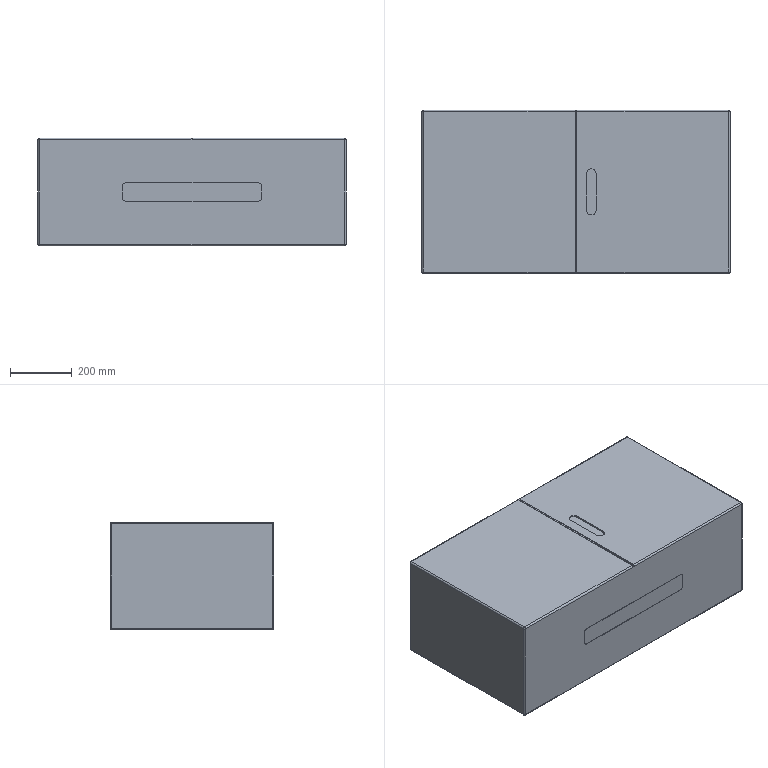Part | SolidWorks | features ICE 3, Fillet 2, Cut 1, Extrusion 1 | 1 solid | 44 faces | box 1000 x 530 x 350 mm | volume 185406118 mm3 | plane 18 | cylinder 18 | sphere 8 | commonest cylinder face diameters 10 x12 20 x4 30 x2
STEP:
#1=CARTESIAN_POINT('',(35.,60.,350.));
#2=VERTEX_POINT('',#1);
#3=CARTESIAN_POINT('',(35.,-60.,350.));
#4=VERTEX_POINT('',#3);
#5=CARTESIAN_POINT('',(35.,60.,350.));
#6=DIRECTION('',(0.,-1.,0.));
#7=VECTOR('',#6,1000.);
#8=LINE('',#5,#7);
#9=EDGE_CURVE('',#2,#4,#8,.T.);
#10=ORIENTED_EDGE('',*,*,#9,.F.);
#11=CARTESIAN_POINT('',(65.,60.,350.));
#12=VERTEX_POINT('',#11);
#13=CARTESIAN_POINT('',(50.,60.,350.));
#14=DIRECTION('',(0.,0.,1.));
#15=DIRECTION('',(1.,0.,0.));
#16=AXIS2_PLACEMENT_3D('',#13,#14,#15);
#17=CIRCLE('',#16,15.);
#18=EDGE_CURVE('',#12,#2,#17,.T.);
#19=ORIENTED_EDGE('',*,*,#18,.F.);
#20=CARTESIAN_POINT('',(65.,-60.,350.));
#21=VERTEX_POINT('',#20);
#22=CARTESIAN_POINT('',(65.,60.,350.));
#23=DIRECTION('',(0.,1.,0.));
#24=VECTOR('',#23,1000.);
#25=LINE('',#22,#24);
#26=EDGE_CURVE('',#21,#12,#25,.T.);
#27=ORIENTED_EDGE('',*,*,#26,.F.);
#28=CARTESIAN_POINT('',(50.,-60.,350.));
#29=DIRECTION('',(0.,0.,1.));
#30=DIRECTION('',(1.,0.,0.));
#31=AXIS2_PLACEMENT_3D('',#28,#29,#30);
#32=CIRCLE('',#31,15.);
#33=EDGE_CURVE('',#4,#21,#32,.T.);
#34=ORIENTED_EDGE('',*,*,#33,.F.);
#35=EDGE_LOOP('',(#10,#19,#27,#34));
#36=FACE_BOUND('',#35,.T.);
#37=CARTESIAN_POINT('',(495.,260.,350.));
#38=VERTEX_POINT('',#37);
#39=CARTESIAN_POINT('',(2.5,260.,350.));
#40=VERTEX_POINT('',#39);
#41=CARTESIAN_POINT('',(500.,260.,350.));
#42=DIRECTION('',(-1.,0.,0.));
#43=VECTOR('',#42,1000.);
#44=LINE('',#41,#43);
#45=EDGE_CURVE('',#38,#40,#44,.T.);
#46=ORIENTED_EDGE('',*,*,#45,.T.);
#47=CARTESIAN_POINT('',(2.5,-260.,350.));
#48=VERTEX_POINT('',#47);
#49=CARTESIAN_POINT('',(2.5,-265.,350.));
#50=DIRECTION('',(0.,1.,0.));
#51=VECTOR('',#50,1000.);
#52=LINE('',#49,#51);
#53=EDGE_CURVE('',#48,#40,#52,.T.);
#54=ORIENTED_EDGE('',*,*,#53,.F.);
#55=CARTESIAN_POINT('',(495.,-260.,350.));
#56=VERTEX_POINT('',#55);
#57=CARTESIAN_POINT('',(500.,-260.,350.));
#58=DIRECTION('',(1.,0.,0.));
#59=VECTOR('',#58,1000.);
#60=LINE('',#57,#59);
#61=EDGE_CURVE('',#48,#56,#60,.T.);
#62=ORIENTED_EDGE('',*,*,#61,.T.);
#63=CARTESIAN_POINT('',(495.,265.,350.));
#64=DIRECTION('',(0.,1.,0.));
#65=VECTOR('',#64,1000.);
#66=LINE('',#63,#65);
#67=EDGE_CURVE('',#56,#38,#66,.T.);
#68=ORIENTED_EDGE('',*,*,#67,.T.);
#69=EDGE_LOOP('',(#46,#54,#62,#68));
#70=FACE_OUTER_BOUND('',#69,.T.);
#71=CARTESIAN_POINT('',(500.,265.,350.));
#72=DIRECTION('',(0.,0.,-1.));
#73=DIRECTION('',(-1.,0.,0.));
#74=AXIS2_PLACEMENT_3D('',#71,#72,#73);
#75=PLANE('',#74);
#76=ADVANCED_FACE('',(#36,#70),#75,.F.);
#77=CARTESIAN_POINT('',(500.,-260.,5.));
#78=VERTEX_POINT('',#77);
#79=CARTESIAN_POINT('',(500.,260.,5.));
#80=VERTEX_POINT('',#79);
#81=CARTESIAN_POINT('',(500.,265.,5.));
#82=DIRECTION('',(0.,1.,0.));
#83=VECTOR('',#82,1000.);
#84=LINE('',#81,#83);
#85=EDGE_CURVE('',#78,#80,#84,.T.);
#86=ORIENTED_EDGE('',*,*,#85,.T.);
#87=CARTESIAN_POINT('',(500.,260.,345.));
#88=VERTEX_POINT('',#87);
#89=CARTESIAN_POINT('',(500.,260.,350.));
#90=DIRECTION('',(0.,0.,1.));
#91=VECTOR('',#90,1000.);
#92=LINE('',#89,#91);
#93=EDGE_CURVE('',#80,#88,#92,.T.);
#94=ORIENTED_EDGE('',*,*,#93,.T.);
#95=CARTESIAN_POINT('',(500.,-260.,345.));
#96=VERTEX_POINT('',#95);
#97=CARTESIAN_POINT('',(500.,-265.,345.));
#98=DIRECTION('',(0.,-1.,0.));
#99=VECTOR('',#98,1000.);
#100=LINE('',#97,#99);
#101=EDGE_CURVE('',#88,#96,#100,.T.);
#102=ORIENTED_EDGE('',*,*,#101,.T.);
#103=CARTESIAN_POINT('',(500.,-260.,350.));
#104=DIRECTION('',(0.,0.,-1.));
#105=VECTOR('',#104,1000.);
#106=LINE('',#103,#105);
#107=EDGE_CURVE('',#96,#78,#106,.T.);
#108=ORIENTED_EDGE('',*,*,#107,.T.);
#109=EDGE_LOOP('',(#86,#94,#102,#108));
#110=FACE_OUTER_BOUND('',#109,.T.);
#111=CARTESIAN_POINT('',(500.,-265.,350.));
#112=DIRECTION('',(-1.,0.,0.));
#113=DIRECTION('',(0.,0.,1.));
#114=AXIS2_PLACEMENT_3D('',#111,#112,#113);
#115=PLANE('',#114);
#116=ADVANCED_FACE('',(#110),#115,.F.);
#117=CARTESIAN_POINT('',(495.,265.,5.));
#118=VERTEX_POINT('',#117);
#119=CARTESIAN_POINT('',(-495.,265.,5.));
#120=VERTEX_POINT('',#119);
#121=CARTESIAN_POINT('',(-500.,265.,5.));
#122=DIRECTION('',(-1.,0.,0.));
#123=VECTOR('',#122,1000.);
#124=LINE('',#121,#123);
#125=EDGE_CURVE('',#118,#120,#124,.T.);
#126=ORIENTED_EDGE('',*,*,#125,.T.);
#127=CARTESIAN_POINT('',(-495.,265.,345.));
#128=VERTEX_POINT('',#127);
#129=CARTESIAN_POINT('',(-495.,265.,350.));
#130=DIRECTION('',(0.,0.,1.));
#131=VECTOR('',#130,1000.);
#132=LINE('',#129,#131);
#133=EDGE_CURVE('',#120,#128,#132,.T.);
#134=ORIENTED_EDGE('',*,*,#133,.T.);
#135=CARTESIAN_POINT('',(495.,265.,345.));
#136=VERTEX_POINT('',#135);
#137=CARTESIAN_POINT('',(-500.,265.,345.));
#138=DIRECTION('',(1.,0.,0.));
#139=VECTOR('',#138,1000.);
#140=LINE('',#137,#139);
#141=EDGE_CURVE('',#128,#136,#140,.T.);
#142=ORIENTED_EDGE('',*,*,#141,.T.);
#143=CARTESIAN_POINT('',(495.,265.,350.));
#144=DIRECTION('',(0.,0.,-1.));
#145=VECTOR('',#144,1000.);
#146=LINE('',#143,#145);
#147=EDGE_CURVE('',#136,#118,#146,.T.);
#148=ORIENTED_EDGE('',*,*,#147,.T.);
#149=EDGE_LOOP('',(#126,#134,#142,#148));
#150=FACE_OUTER_BOUND('',#149,.T.);
#151=CARTESIAN_POINT('',(-500.,265.,350.));
#152=DIRECTION('',(0.,-1.,0.));
#153=DIRECTION('',(0.,0.,-1.));
#154=AXIS2_PLACEMENT_3D('',#151,#152,#153);
#155=PLANE('',#154);
#156=ADVANCED_FACE('',(#150),#155,.F.);
#157=CARTESIAN_POINT('',(-500.,-260.,345.));
#158=VERTEX_POINT('',#157);
#159=CARTESIAN_POINT('',(-500.,260.,345.));
#160=VERTEX_POINT('',#159);
#161=CARTESIAN_POINT('',(-500.,-265.,345.));
#162=DIRECTION('',(0.,1.,0.));
#163=VECTOR('',#162,1000.);
#164=LINE('',#161,#163);
#165=EDGE_CURVE('',#158,#160,#164,.T.);
#166=ORIENTED_EDGE('',*,*,#165,.T.);
#167=CARTESIAN_POINT('',(-500.,260.,5.));
#168=VERTEX_POINT('',#167);
#169=CARTESIAN_POINT('',(-500.,260.,350.));
#170=DIRECTION('',(0.,0.,-1.));
#171=VECTOR('',#170,1000.);
#172=LINE('',#169,#171);
#173=EDGE_CURVE('',#160,#168,#172,.T.);
#174=ORIENTED_EDGE('',*,*,#173,.T.);
#175=CARTESIAN_POINT('',(-500.,-260.,5.));
#176=VERTEX_POINT('',#175);
#177=CARTESIAN_POINT('',(-500.,-265.,5.));
#178=DIRECTION('',(0.,-1.,0.));
#179=VECTOR('',#178,1000.);
#180=LINE('',#177,#179);
#181=EDGE_CURVE('',#168,#176,#180,.T.);
#182=ORIENTED_EDGE('',*,*,#181,.T.);
#183=CARTESIAN_POINT('',(-500.,-260.,350.));
#184=DIRECTION('',(0.,0.,1.));
#185=VECTOR('',#184,1000.);
#186=LINE('',#183,#185);
#187=EDGE_CURVE('',#176,#158,#186,.T.);
#188=ORIENTED_EDGE('',*,*,#187,.T.);
#189=EDGE_LOOP('',(#166,#174,#182,#188));
#190=FACE_OUTER_BOUND('',#189,.T.);
#191=CARTESIAN_POINT('',(-500.,-265.,350.));
#192=DIRECTION('',(1.,0.,0.));
#193=DIRECTION('',(0.,0.,-1.));
#194=AXIS2_PLACEMENT_3D('',#191,#192,#193);
#195=PLANE('',#194);
#196=ADVANCED_FACE('',(#190),#195,.F.);
#197=CARTESIAN_POINT('',(215.,-265.,205.));
#198=VERTEX_POINT('',#197);
#199=CARTESIAN_POINT('',(-215.,-265.,205.));
#200=VERTEX_POINT('',#199);
#201=CARTESIAN_POINT('',(-225.,-265.,205.));
#202=DIRECTION('',(-1.,0.,0.));
#203=VECTOR('',#202,1000.);
#204=LINE('',#201,#203);
#205=EDGE_CURVE('',#198,#200,#204,.T.);
#206=ORIENTED_EDGE('',*,*,#205,.F.);
#207=CARTESIAN_POINT('',(225.,-265.,195.));
#208=VERTEX_POINT('',#207);
#209=CARTESIAN_POINT('',(215.,-265.,195.));
#210=DIRECTION('',(0.,1.,0.));
#211=DIRECTION('',(0.,0.,1.));
#212=AXIS2_PLACEMENT_3D('',#209,#210,#211);
#213=CIRCLE('',#212,10.);
#214=EDGE_CURVE('',#198,#208,#213,.T.);
#215=ORIENTED_EDGE('',*,*,#214,.T.);
#216=CARTESIAN_POINT('',(225.,-265.,155.));
#217=VERTEX_POINT('',#216);
#218=CARTESIAN_POINT('',(225.,-265.,145.));
#219=DIRECTION('',(0.,0.,1.));
#220=VECTOR('',#219,1000.);
#221=LINE('',#218,#220);
#222=EDGE_CURVE('',#217,#208,#221,.T.);
#223=ORIENTED_EDGE('',*,*,#222,.F.);
#224=CARTESIAN_POINT('',(215.,-265.,145.));
#225=VERTEX_POINT('',#224);
#226=CARTESIAN_POINT('',(215.,-265.,155.));
#227=DIRECTION('',(0.,1.,0.));
#228=DIRECTION('',(0.,0.,1.));
#229=AXIS2_PLACEMENT_3D('',#226,#227,#228);
#230=CIRCLE('',#229,10.);
#231=EDGE_CURVE('',#217,#225,#230,.T.);
#232=ORIENTED_EDGE('',*,*,#231,.T.);
#233=CARTESIAN_POINT('',(-215.,-265.,145.));
#234=VERTEX_POINT('',#233);
#235=CARTESIAN_POINT('',(-225.,-265.,145.));
#236=DIRECTION('',(1.,0.,0.));
#237=VECTOR('',#236,1000.);
#238=LINE('',#235,#237);
#239=EDGE_CURVE('',#234,#225,#238,.T.);
#240=ORIENTED_EDGE('',*,*,#239,.F.);
#241=CARTESIAN_POINT('',(-225.,-265.,155.));
#242=VERTEX_POINT('',#241);
#243=CARTESIAN_POINT('',(-215.,-265.,155.));
#244=DIRECTION('',(0.,1.,0.));
#245=DIRECTION('',(0.,0.,1.));
#246=AXIS2_PLACEMENT_3D('',#243,#244,#245);
#247=CIRCLE('',#246,10.);
#248=EDGE_CURVE('',#234,#242,#247,.T.);
#249=ORIENTED_EDGE('',*,*,#248,.T.);
#250=CARTESIAN_POINT('',(-225.,-265.,195.));
#251=VERTEX_POINT('',#250);
#252=CARTESIAN_POINT('',(-225.,-265.,145.));
#253=DIRECTION('',(0.,0.,-1.));
#254=VECTOR('',#253,1000.);
#255=LINE('',#252,#254);
#256=EDGE_CURVE('',#251,#242,#255,.T.);
#257=ORIENTED_EDGE('',*,*,#256,.F.);
#258=CARTESIAN_POINT('',(-215.,-265.,195.));
#259=DIRECTION('',(0.,1.,0.));
#260=DIRECTION('',(0.,0.,1.));
#261=AXIS2_PLACEMENT_3D('',#258,#259,#260);
#262=CIRCLE('',#261,10.);
#263=EDGE_CURVE('',#251,#200,#262,.T.);
#264=ORIENTED_EDGE('',*,*,#263,.T.);
#265=EDGE_LOOP('',(#206,#215,#223,#232,#240,#249,#257,#264));
#266=FACE_BOUND('',#265,.T.);
#267=CARTESIAN_POINT('',(495.,-265.,345.));
#268=VERTEX_POINT('',#267);
#269=CARTESIAN_POINT('',(-495.,-265.,345.));
#270=VERTEX_POINT('',#269);
#271=CARTESIAN_POINT('',(-500.,-265.,345.));
#272=DIRECTION('',(-1.,0.,0.));
#273=VECTOR('',#272,1000.);
#274=LINE('',#271,#273);
#275=EDGE_CURVE('',#268,#270,#274,.T.);
#276=ORIENTED_EDGE('',*,*,#275,.T.);
#277=CARTESIAN_POINT('',(-495.,-265.,5.));
#278=VERTEX_POINT('',#277);
#279=CARTESIAN_POINT('',(-495.,-265.,350.));
#280=DIRECTION('',(0.,0.,-1.));
#281=VECTOR('',#280,1000.);
#282=LINE('',#279,#281);
#283=EDGE_CURVE('',#270,#278,#282,.T.);
#284=ORIENTED_EDGE('',*,*,#283,.T.);
#285=CARTESIAN_POINT('',(495.,-265.,5.));
#286=VERTEX_POINT('',#285);
#287=CARTESIAN_POINT('',(500.,-265.,5.));
#288=DIRECTION('',(1.,0.,0.));
#289=VECTOR('',#288,1000.);
#290=LINE('',#287,#289);
#291=EDGE_CURVE('',#278,#286,#290,.T.);
#292=ORIENTED_EDGE('',*,*,#291,.T.);
#293=CARTESIAN_POINT('',(495.,-265.,350.));
#294=DIRECTION('',(0.,0.,1.));
#295=VECTOR('',#294,1000.);
#296=LINE('',#293,#295);
#297=EDGE_CURVE('',#286,#268,#296,.T.);
#298=ORIENTED_EDGE('',*,*,#297,.T.);
#299=EDGE_LOOP('',(#276,#284,#292,#298));
#300=FACE_OUTER_BOUND('',#299,.T.);
#301=CARTESIAN_POINT('',(-500.,-265.,350.));
#302=DIRECTION('',(0.,1.,0.));
#303=DIRECTION('',(0.,0.,1.));
#304=AXIS2_PLACEMENT_3D('',#301,#302,#303);
#305=PLANE('',#304);
#306=ADVANCED_FACE('',(#266,#300),#305,.F.);
#307=CARTESIAN_POINT('',(-495.,-260.,350.));
#308=VERTEX_POINT('',#307);
#309=CARTESIAN_POINT('',(-2.5,-260.,350.));
#310=VERTEX_POINT('',#309);
#311=CARTESIAN_POINT('',(500.,-260.,350.));
#312=DIRECTION('',(1.,0.,0.));
#313=VECTOR('',#312,1000.);
#314=LINE('',#311,#313);
#315=EDGE_CURVE('',#308,#310,#314,.T.);
#316=ORIENTED_EDGE('',*,*,#315,.T.);
#317=CARTESIAN_POINT('',(-2.5,260.,350.));
#318=VERTEX_POINT('',#317);
#319=CARTESIAN_POINT('',(-2.5,-265.,350.));
#320=DIRECTION('',(0.,-1.,0.));
#321=VECTOR('',#320,1000.);
#322=LINE('',#319,#321);
#323=EDGE_CURVE('',#318,#310,#322,.T.);
#324=ORIENTED_EDGE('',*,*,#323,.F.);
#325=CARTESIAN_POINT('',(-495.,260.,350.));
#326=VERTEX_POINT('',#325);
#327=CARTESIAN_POINT('',(500.,260.,350.));
#328=DIRECTION('',(-1.,0.,0.));
#329=VECTOR('',#328,1000.);
#330=LINE('',#327,#329);
#331=EDGE_CURVE('',#318,#326,#330,.T.);
#332=ORIENTED_EDGE('',*,*,#331,.T.);
#333=CARTESIAN_POINT('',(-495.,265.,350.));
#334=DIRECTION('',(0.,-1.,0.));
#335=VECTOR('',#334,1000.);
#336=LINE('',#333,#335);
#337=EDGE_CURVE('',#326,#308,#336,.T.);
#338=ORIENTED_EDGE('',*,*,#337,.T.);
#339=EDGE_LOOP('',(#316,#324,#332,#338));
#340=FACE_OUTER_BOUND('',#339,.T.);
#341=CARTESIAN_POINT('',(500.,265.,350.));
#342=DIRECTION('',(0.,0.,-1.));
#343=DIRECTION('',(-1.,0.,0.));
#344=AXIS2_PLACEMENT_3D('',#341,#342,#343);
#345=PLANE('',#344);
#346=ADVANCED_FACE('',(#340),#345,.F.);
#347=CARTESIAN_POINT('',(-495.,-260.,0.));
#348=VERTEX_POINT('',#347);
#349=CARTESIAN_POINT('',(-495.,260.,0.));
#350=VERTEX_POINT('',#349);
#351=CARTESIAN_POINT('',(-495.,265.,0.));
#352=DIRECTION('',(0.,1.,0.));
#353=VECTOR('',#352,1000.);
#354=LINE('',#351,#353);
#355=EDGE_CURVE('',#348,#350,#354,.T.);
#356=ORIENTED_EDGE('',*,*,#355,.T.);
#357=CARTESIAN_POINT('',(495.,260.,0.));
#358=VERTEX_POINT('',#357);
#359=CARTESIAN_POINT('',(500.,260.,0.));
#360=DIRECTION('',(1.,0.,0.));
#361=VECTOR('',#360,1000.);
#362=LINE('',#359,#361);
#363=EDGE_CURVE('',#350,#358,#362,.T.);
#364=ORIENTED_EDGE('',*,*,#363,.T.);
#365=CARTESIAN_POINT('',(495.,-260.,0.));
#366=VERTEX_POINT('',#365);
#367=CARTESIAN_POINT('',(495.,-265.,0.));
#368=DIRECTION('',(0.,-1.,0.));
#369=VECTOR('',#368,1000.);
#370=LINE('',#367,#369);
#371=EDGE_CURVE('',#358,#366,#370,.T.);
#372=ORIENTED_EDGE('',*,*,#371,.T.);
#373=CARTESIAN_POINT('',(-500.,-260.,0.));
#374=DIRECTION('',(-1.,0.,0.));
#375=VECTOR('',#374,1000.);
#376=LINE('',#373,#375);
#377=EDGE_CURVE('',#366,#348,#376,.T.);
#378=ORIENTED_EDGE('',*,*,#377,.T.);
#379=EDGE_LOOP('',(#356,#364,#372,#378));
#380=FACE_OUTER_BOUND('',#379,.T.);
#381=CARTESIAN_POINT('',(500.,265.,0.));
#382=DIRECTION('',(0.,0.,-1.));
#383=DIRECTION('',(-1.,0.,0.));
#384=AXIS2_PLACEMENT_3D('',#381,#382,#383);
#385=PLANE('',#384);
#386=ADVANCED_FACE('',(#380),#385,.T.);
#387=CARTESIAN_POINT('',(2.5,-264.,348.));
#388=VERTEX_POINT('',#387);
#389=CARTESIAN_POINT('',(2.5,-260.,345.));
#390=DIRECTION('',(-1.,0.,0.));
#391=DIRECTION('',(0.,0.,-1.));
#392=AXIS2_PLACEMENT_3D('',#389,#390,#391);
#393=CIRCLE('',#392,5.);
#394=EDGE_CURVE('',#388,#48,#393,.T.);
#395=ORIENTED_EDGE('',*,*,#394,.F.);
#396=CARTESIAN_POINT('',(-2.5,-264.,348.));
#397=VERTEX_POINT('',#396);
#398=CARTESIAN_POINT('',(500.,-264.,348.));
#399=DIRECTION('',(1.,0.,0.));
#400=VECTOR('',#399,1000.);
#401=LINE('',#398,#400);
#402=EDGE_CURVE('',#397,#388,#401,.T.);
#403=ORIENTED_EDGE('',*,*,#402,.F.);
#404=CARTESIAN_POINT('',(-2.5,-260.,345.));
#405=DIRECTION('',(1.,0.,0.));
#406=DIRECTION('',(0.,0.,1.));
#407=AXIS2_PLACEMENT_3D('',#404,#405,#406);
#408=CIRCLE('',#407,5.);
#409=EDGE_CURVE('',#310,#397,#408,.T.);
#410=ORIENTED_EDGE('',*,*,#409,.F.);
#411=ORIENTED_EDGE('',*,*,#315,.F.);
#412=CARTESIAN_POINT('',(-495.,-260.,345.));
#413=DIRECTION('',(-1.,0.,0.));
#414=DIRECTION('',(0.,0.,1.));
#415=AXIS2_PLACEMENT_3D('',#412,#413,#414);
#416=CIRCLE('',#415,5.);
#417=EDGE_CURVE('',#270,#308,#416,.T.);
#418=ORIENTED_EDGE('',*,*,#417,.F.);
#419=ORIENTED_EDGE('',*,*,#275,.F.);
#420=CARTESIAN_POINT('',(495.,-260.,345.));
#421=DIRECTION('',(1.,0.,0.));
#422=DIRECTION('',(0.,0.,-1.));
#423=AXIS2_PLACEMENT_3D('',#420,#421,#422);
#424=CIRCLE('',#423,5.);
#425=EDGE_CURVE('',#56,#268,#424,.T.);
#426=ORIENTED_EDGE('',*,*,#425,.F.);
#427=ORIENTED_EDGE('',*,*,#61,.F.);
#428=EDGE_LOOP('',(#395,#403,#410,#411,#418,#419,#426,#427));
#429=FACE_OUTER_BOUND('',#428,.T.);
#430=CARTESIAN_POINT('',(500.,-260.,345.));
#431=DIRECTION('',(1.,0.,0.));
#432=DIRECTION('',(0.,0.,-1.));
#433=AXIS2_PLACEMENT_3D('',#430,#431,#432);
#434=CYLINDRICAL_SURFACE('',#433,5.);
#435=ADVANCED_FACE('',(#429),#434,.T.);
#436=CARTESIAN_POINT('',(495.,-260.,345.));
#437=DIRECTION('',(0.,1.,0.));
#438=DIRECTION('',(0.,0.,-1.));
#439=AXIS2_PLACEMENT_3D('',#436,#437,#438);
#440=CIRCLE('',#439,5.);
#441=EDGE_CURVE('',#56,#96,#440,.T.);
#442=ORIENTED_EDGE('',*,*,#441,.F.);
#443=ORIENTED_EDGE('',*,*,#425,.T.);
#444=CARTESIAN_POINT('',(495.,-260.,345.));
#445=DIRECTION('',(0.,0.,-1.));
#446=DIRECTION('',(1.,0.,0.));
#447=AXIS2_PLACEMENT_3D('',#444,#445,#446);
#448=CIRCLE('',#447,5.);
#449=EDGE_CURVE('',#96,#268,#448,.T.);
#450=ORIENTED_EDGE('',*,*,#449,.F.);
#451=EDGE_LOOP('',(#442,#443,#450));
#452=FACE_OUTER_BOUND('',#451,.T.);
#453=CARTESIAN_POINT('',(495.,-260.,345.));
#454=DIRECTION('',(0.,1.,0.));
#455=DIRECTION('',(1.,0.,0.));
#456=AXIS2_PLACEMENT_3D('',#453,#454,#455);
#457=SPHERICAL_SURFACE('',#456,5.);
#458=ADVANCED_FACE('',(#452),#457,.T.);
#459=CARTESIAN_POINT('',(-495.,-260.,345.));
#460=DIRECTION('',(0.,0.,-1.));
#461=DIRECTION('',(1.,0.,0.));
#462=AXIS2_PLACEMENT_3D('',#459,#460,#461);
#463=CIRCLE('',#462,5.);
#464=EDGE_CURVE('',#270,#158,#463,.T.);
#465=ORIENTED_EDGE('',*,*,#464,.F.);
#466=ORIENTED_EDGE('',*,*,#417,.T.);
#467=CARTESIAN_POINT('',(-495.,-260.,345.));
#468=DIRECTION('',(0.,1.,0.));
#469=DIRECTION('',(0.,0.,-1.));
#470=AXIS2_PLACEMENT_3D('',#467,#468,#469);
#471=CIRCLE('',#470,5.);
#472=EDGE_CURVE('',#158,#308,#471,.T.);
#473=ORIENTED_EDGE('',*,*,#472,.F.);
#474=EDGE_LOOP('',(#465,#466,#473));
#475=FACE_OUTER_BOUND('',#474,.T.);
#476=CARTESIAN_POINT('',(-495.,-260.,345.));
#477=DIRECTION('',(0.,1.,0.));
#478=DIRECTION('',(1.,0.,0.));
#479=AXIS2_PLACEMENT_3D('',#476,#477,#478);
#480=SPHERICAL_SURFACE('',#479,5.);
#481=ADVANCED_FACE('',(#475),#480,.T.);
#482=ORIENTED_EDGE('',*,*,#449,.T.);
#483=ORIENTED_EDGE('',*,*,#297,.F.);
#484=CARTESIAN_POINT('',(495.,-260.,5.));
#485=DIRECTION('',(0.,0.,-1.));
#486=DIRECTION('',(-1.,0.,0.));
#487=AXIS2_PLACEMENT_3D('',#484,#485,#486);
#488=CIRCLE('',#487,5.);
#489=EDGE_CURVE('',#78,#286,#488,.T.);
#490=ORIENTED_EDGE('',*,*,#489,.F.);
#491=ORIENTED_EDGE('',*,*,#107,.F.);
#492=EDGE_LOOP('',(#482,#483,#490,#491));
#493=FACE_OUTER_BOUND('',#492,.T.);
#494=CARTESIAN_POINT('',(495.,-260.,350.));
#495=DIRECTION('',(0.,0.,-1.));
#496=DIRECTION('',(-1.,0.,0.));
#497=AXIS2_PLACEMENT_3D('',#494,#495,#496);
#498=CYLINDRICAL_SURFACE('',#497,5.);
#499=ADVANCED_FACE('',(#493),#498,.T.);
#500=ORIENTED_EDGE('',*,*,#441,.T.);
#501=ORIENTED_EDGE('',*,*,#101,.F.);
#502=CARTESIAN_POINT('',(495.,260.,345.));
#503=DIRECTION('',(0.,1.,0.));
#504=DIRECTION('',(0.,0.,1.));
#505=AXIS2_PLACEMENT_3D('',#502,#503,#504);
#506=CIRCLE('',#505,5.);
#507=EDGE_CURVE('',#38,#88,#506,.T.);
#508=ORIENTED_EDGE('',*,*,#507,.F.);
#509=ORIENTED_EDGE('',*,*,#67,.F.);
#510=EDGE_LOOP('',(#500,#501,#508,#509));
#511=FACE_OUTER_BOUND('',#510,.T.);
#512=CARTESIAN_POINT('',(495.,265.,345.));
#513=DIRECTION('',(0.,1.,0.));
#514=DIRECTION('',(0.,0.,1.));
#515=AXIS2_PLACEMENT_3D('',#512,#513,#514);
#516=CYLINDRICAL_SURFACE('',#515,5.);
#517=ADVANCED_FACE('',(#511),#516,.T.);
#518=CARTESIAN_POINT('',(2.5,264.,348.));
#519=VERTEX_POINT('',#518);
#520=CARTESIAN_POINT('',(2.5,260.,345.));
#521=DIRECTION('',(-1.,0.,0.));
#522=DIRECTION('',(0.,0.,-1.));
#523=AXIS2_PLACEMENT_3D('',#520,#521,#522);
#524=CIRCLE('',#523,5.);
#525=EDGE_CURVE('',#40,#519,#524,.T.);
#526=ORIENTED_EDGE('',*,*,#525,.F.);
#527=ORIENTED_EDGE('',*,*,#45,.F.);
#528=CARTESIAN_POINT('',(495.,260.,345.));
#529=DIRECTION('',(1.,0.,0.));
#530=DIRECTION('',(0.,0.,-1.));
#531=AXIS2_PLACEMENT_3D('',#528,#529,#530);
#532=CIRCLE('',#531,5.);
#533=EDGE_CURVE('',#136,#38,#532,.T.);
#534=ORIENTED_EDGE('',*,*,#533,.F.);
#535=ORIENTED_EDGE('',*,*,#141,.F.);
#536=CARTESIAN_POINT('',(-495.,260.,345.));
#537=DIRECTION('',(-1.,0.,0.));
#538=DIRECTION('',(0.,-1.,0.));
#539=AXIS2_PLACEMENT_3D('',#536,#537,#538);
#540=CIRCLE('',#539,5.);
#541=EDGE_CURVE('',#326,#128,#540,.T.);
#542=ORIENTED_EDGE('',*,*,#541,.F.);
#543=ORIENTED_EDGE('',*,*,#331,.F.);
#544=CARTESIAN_POINT('',(-2.5,264.,348.));
#545=VERTEX_POINT('',#544);
#546=CARTESIAN_POINT('',(-2.5,260.,345.));
#547=DIRECTION('',(1.,0.,0.));
#548=DIRECTION('',(0.,0.,1.));
#549=AXIS2_PLACEMENT_3D('',#546,#547,#548);
#550=CIRCLE('',#549,5.);
#551=EDGE_CURVE('',#545,#318,#550,.T.);
#552=ORIENTED_EDGE('',*,*,#551,.F.);
#553=CARTESIAN_POINT('',(500.,264.,348.));
#554=DIRECTION('',(-1.,0.,0.));
#555=VECTOR('',#554,1000.);
#556=LINE('',#553,#555);
#557=EDGE_CURVE('',#519,#545,#556,.T.);
#558=ORIENTED_EDGE('',*,*,#557,.F.);
#559=EDGE_LOOP('',(#526,#527,#534,#535,#542,#543,#552,#558));
#560=FACE_OUTER_BOUND('',#559,.T.);
#561=CARTESIAN_POINT('',(500.,260.,345.));
#562=DIRECTION('',(-1.,0.,0.));
#563=DIRECTION('',(0.,0.,1.));
#564=AXIS2_PLACEMENT_3D('',#561,#562,#563);
#565=CYLINDRICAL_SURFACE('',#564,5.);
#566=ADVANCED_FACE('',(#560),#565,.T.);
#567=ORIENTED_EDGE('',*,*,#472,.T.);
#568=ORIENTED_EDGE('',*,*,#337,.F.);
#569=CARTESIAN_POINT('',(-495.,260.,345.));
#570=DIRECTION('',(0.,1.,0.));
#571=DIRECTION('',(0.,0.,1.));
#572=AXIS2_PLACEMENT_3D('',#569,#570,#571);
#573=CIRCLE('',#572,5.);
#574=EDGE_CURVE('',#160,#326,#573,.T.);
#575=ORIENTED_EDGE('',*,*,#574,.F.);
#576=ORIENTED_EDGE('',*,*,#165,.F.);
#577=EDGE_LOOP('',(#567,#568,#575,#576));
#578=FACE_OUTER_BOUND('',#577,.T.);
#579=CARTESIAN_POINT('',(-495.,265.,345.));
#580=DIRECTION('',(0.,-1.,0.));
#581=DIRECTION('',(0.,0.,-1.));
#582=AXIS2_PLACEMENT_3D('',#579,#580,#581);
#583=CYLINDRICAL_SURFACE('',#582,5.);
#584=ADVANCED_FACE('',(#578),#583,.T.);
#585=ORIENTED_EDGE('',*,*,#464,.T.);
#586=ORIENTED_EDGE('',*,*,#187,.F.);
#587=CARTESIAN_POINT('',(-495.,-260.,5.));
#588=DIRECTION('',(0.,0.,-1.));
#589=DIRECTION('',(-1.,0.,0.));
#590=AXIS2_PLACEMENT_3D('',#587,#588,#589);
#591=CIRCLE('',#590,5.);
#592=EDGE_CURVE('',#278,#176,#591,.T.);
#593=ORIENTED_EDGE('',*,*,#592,.F.);
#594=ORIENTED_EDGE('',*,*,#283,.F.);
#595=EDGE_LOOP('',(#585,#586,#593,#594));
#596=FACE_OUTER_BOUND('',#595,.T.);
#597=CARTESIAN_POINT('',(-495.,-260.,350.));
#598=DIRECTION('',(0.,0.,-1.));
#599=DIRECTION('',(-1.,0.,0.));
#600=AXIS2_PLACEMENT_3D('',#597,#598,#599);
#601=CYLINDRICAL_SURFACE('',#600,5.);
#602=ADVANCED_FACE('',(#596),#601,.T.);
#603=CARTESIAN_POINT('',(495.,-260.,5.));
#604=DIRECTION('',(1.,0.,0.));
#605=DIRECTION('',(0.,0.,-1.));
#606=AXIS2_PLACEMENT_3D('',#603,#604,#605);
#607=CIRCLE('',#606,5.);
#608=EDGE_CURVE('',#286,#366,#607,.T.);
#609=ORIENTED_EDGE('',*,*,#608,.F.);
#610=ORIENTED_EDGE('',*,*,#291,.F.);
#611=CARTESIAN_POINT('',(-495.,-260.,5.));
#612=DIRECTION('',(-1.,0.,0.));
#613=DIRECTION('',(0.,0.,1.));
#614=AXIS2_PLACEMENT_3D('',#611,#612,#613);
#615=CIRCLE('',#614,5.);
#616=EDGE_CURVE('',#348,#278,#615,.T.);
#617=ORIENTED_EDGE('',*,*,#616,.F.);
#618=ORIENTED_EDGE('',*,*,#377,.F.);
#619=EDGE_LOOP('',(#609,#610,#617,#618));
#620=FACE_OUTER_BOUND('',#619,.T.);
#621=CARTESIAN_POINT('',(-500.,-260.,5.));
#622=DIRECTION('',(-1.,0.,0.));
#623=DIRECTION('',(0.,0.,1.));
#624=AXIS2_PLACEMENT_3D('',#621,#622,#623);
#625=CYLINDRICAL_SURFACE('',#624,5.);
#626=ADVANCED_FACE('',(#620),#625,.T.);
#627=ORIENTED_EDGE('',*,*,#489,.T.);
#628=ORIENTED_EDGE('',*,*,#608,.T.);
#629=CARTESIAN_POINT('',(495.,-260.,5.));
#630=DIRECTION('',(0.,1.,0.));
#631=DIRECTION('',(0.,0.,-1.));
#632=AXIS2_PLACEMENT_3D('',#629,#630,#631);
#633=CIRCLE('',#632,5.);
#634=EDGE_CURVE('',#78,#366,#633,.T.);
#635=ORIENTED_EDGE('',*,*,#634,.F.);
#636=EDGE_LOOP('',(#627,#628,#635));
#637=FACE_OUTER_BOUND('',#636,.T.);
#638=CARTESIAN_POINT('',(495.,-260.,5.));
#639=DIRECTION('',(0.,1.,0.));
#640=DIRECTION('',(1.,0.,0.));
#641=AXIS2_PLACEMENT_3D('',#638,#639,#640);
#642=SPHERICAL_SURFACE('',#641,5.);
#643=ADVANCED_FACE('',(#637),#642,.T.);
#644=ORIENTED_EDGE('',*,*,#533,.T.);
#645=ORIENTED_EDGE('',*,*,#507,.T.);
#646=CARTESIAN_POINT('',(495.,260.,345.));
#647=DIRECTION('',(0.,0.,-1.));
#648=DIRECTION('',(1.,0.,0.));
#649=AXIS2_PLACEMENT_3D('',#646,#647,#648);
#650=CIRCLE('',#649,5.);
#651=EDGE_CURVE('',#136,#88,#650,.T.);
#652=ORIENTED_EDGE('',*,*,#651,.F.);
#653=EDGE_LOOP('',(#644,#645,#652));
#654=FACE_OUTER_BOUND('',#653,.T.);
#655=CARTESIAN_POINT('',(495.,260.,345.));
#656=DIRECTION('',(0.,1.,0.));
#657=DIRECTION('',(1.,0.,0.));
#658=AXIS2_PLACEMENT_3D('',#655,#656,#657);
#659=SPHERICAL_SURFACE('',#658,5.);
#660=ADVANCED_FACE('',(#654),#659,.T.);
#661=ORIENTED_EDGE('',*,*,#574,.T.);
#662=ORIENTED_EDGE('',*,*,#541,.T.);
#663=CARTESIAN_POINT('',(-495.,260.,345.));
#664=DIRECTION('',(0.,0.,-1.));
#665=DIRECTION('',(1.,0.,0.));
#666=AXIS2_PLACEMENT_3D('',#663,#664,#665);
#667=CIRCLE('',#666,5.);
#668=EDGE_CURVE('',#160,#128,#667,.T.);
#669=ORIENTED_EDGE('',*,*,#668,.F.);
#670=EDGE_LOOP('',(#661,#662,#669));
#671=FACE_OUTER_BOUND('',#670,.T.);
#672=CARTESIAN_POINT('',(-495.,260.,345.));
#673=DIRECTION('',(0.,1.,0.));
#674=DIRECTION('',(1.,0.,0.));
#675=AXIS2_PLACEMENT_3D('',#672,#673,#674);
#676=SPHERICAL_SURFACE('',#675,5.);
#677=ADVANCED_FACE('',(#671),#676,.T.);
#678=ORIENTED_EDGE('',*,*,#616,.T.);
#679=ORIENTED_EDGE('',*,*,#592,.T.);
#680=CARTESIAN_POINT('',(-495.,-260.,5.));
#681=DIRECTION('',(0.,1.,0.));
#682=DIRECTION('',(0.,0.,-1.));
#683=AXIS2_PLACEMENT_3D('',#680,#681,#682);
#684=CIRCLE('',#683,5.);
#685=EDGE_CURVE('',#348,#176,#684,.T.);
#686=ORIENTED_EDGE('',*,*,#685,.F.);
#687=EDGE_LOOP('',(#678,#679,#686));
#688=FACE_OUTER_BOUND('',#687,.T.);
#689=CARTESIAN_POINT('',(-495.,-260.,5.));
#690=DIRECTION('',(0.,1.,0.));
#691=DIRECTION('',(1.,0.,0.));
#692=AXIS2_PLACEMENT_3D('',#689,#690,#691);
#693=SPHERICAL_SURFACE('',#692,5.);
#694=ADVANCED_FACE('',(#688),#693,.T.);
#695=ORIENTED_EDGE('',*,*,#634,.T.);
#696=ORIENTED_EDGE('',*,*,#371,.F.);
#697=CARTESIAN_POINT('',(495.,260.,5.));
#698=DIRECTION('',(0.,1.,0.));
#699=DIRECTION('',(0.,0.,1.));
#700=AXIS2_PLACEMENT_3D('',#697,#698,#699);
#701=CIRCLE('',#700,5.);
#702=EDGE_CURVE('',#80,#358,#701,.T.);
#703=ORIENTED_EDGE('',*,*,#702,.F.);
#704=ORIENTED_EDGE('',*,*,#85,.F.);
#705=EDGE_LOOP('',(#695,#696,#703,#704));
#706=FACE_OUTER_BOUND('',#705,.T.);
#707=CARTESIAN_POINT('',(495.,-265.,5.));
#708=DIRECTION('',(0.,-1.,0.));
#709=DIRECTION('',(0.,0.,-1.));
#710=AXIS2_PLACEMENT_3D('',#707,#708,#709);
#711=CYLINDRICAL_SURFACE('',#710,5.);
#712=ADVANCED_FACE('',(#706),#711,.T.);
#713=ORIENTED_EDGE('',*,*,#651,.T.);
#714=ORIENTED_EDGE('',*,*,#93,.F.);
#715=CARTESIAN_POINT('',(495.,260.,5.));
#716=DIRECTION('',(0.,0.,-1.));
#717=DIRECTION('',(-1.,0.,0.));
#718=AXIS2_PLACEMENT_3D('',#715,#716,#717);
#719=CIRCLE('',#718,5.);
#720=EDGE_CURVE('',#118,#80,#719,.T.);
#721=ORIENTED_EDGE('',*,*,#720,.F.);
#722=ORIENTED_EDGE('',*,*,#147,.F.);
#723=EDGE_LOOP('',(#713,#714,#721,#722));
#724=FACE_OUTER_BOUND('',#723,.T.);
#725=CARTESIAN_POINT('',(495.,260.,350.));
#726=DIRECTION('',(0.,0.,-1.));
#727=DIRECTION('',(-1.,0.,0.));
#728=AXIS2_PLACEMENT_3D('',#725,#726,#727);
#729=CYLINDRICAL_SURFACE('',#728,5.);
#730=ADVANCED_FACE('',(#724),#729,.T.);
#731=ORIENTED_EDGE('',*,*,#668,.T.);
#732=ORIENTED_EDGE('',*,*,#133,.F.);
#733=CARTESIAN_POINT('',(-495.,260.,5.));
#734=DIRECTION('',(0.,0.,-1.));
#735=DIRECTION('',(-1.,0.,0.));
#736=AXIS2_PLACEMENT_3D('',#733,#734,#735);
#737=CIRCLE('',#736,5.);
#738=EDGE_CURVE('',#168,#120,#737,.T.);
#739=ORIENTED_EDGE('',*,*,#738,.F.);
#740=ORIENTED_EDGE('',*,*,#173,.F.);
#741=EDGE_LOOP('',(#731,#732,#739,#740));
#742=FACE_OUTER_BOUND('',#741,.T.);
#743=CARTESIAN_POINT('',(-495.,260.,350.));
#744=DIRECTION('',(0.,0.,-1.));
#745=DIRECTION('',(-1.,0.,0.));
#746=AXIS2_PLACEMENT_3D('',#743,#744,#745);
#747=CYLINDRICAL_SURFACE('',#746,5.);
#748=ADVANCED_FACE('',(#742),#747,.T.);
#749=ORIENTED_EDGE('',*,*,#685,.T.);
#750=ORIENTED_EDGE('',*,*,#181,.F.);
#751=CARTESIAN_POINT('',(-495.,260.,5.));
#752=DIRECTION('',(0.,1.,0.));
#753=DIRECTION('',(0.,0.,1.));
#754=AXIS2_PLACEMENT_3D('',#751,#752,#753);
#755=CIRCLE('',#754,5.);
#756=EDGE_CURVE('',#350,#168,#755,.T.);
#757=ORIENTED_EDGE('',*,*,#756,.F.);
#758=ORIENTED_EDGE('',*,*,#355,.F.);
#759=EDGE_LOOP('',(#749,#750,#757,#758));
#760=FACE_OUTER_BOUND('',#759,.T.);
#761=CARTESIAN_POINT('',(-495.,-265.,5.));
#762=DIRECTION('',(0.,1.,0.));
#763=DIRECTION('',(0.,0.,1.));
#764=AXIS2_PLACEMENT_3D('',#761,#762,#763);
#765=CYLINDRICAL_SURFACE('',#764,5.);
#766=ADVANCED_FACE('',(#760),#765,.T.);
#767=ORIENTED_EDGE('',*,*,#720,.T.);
#768=ORIENTED_EDGE('',*,*,#702,.T.);
#769=CARTESIAN_POINT('',(495.,260.,5.));
#770=DIRECTION('',(-1.,0.,0.));
#771=DIRECTION('',(0.,1.,0.));
#772=AXIS2_PLACEMENT_3D('',#769,#770,#771);
#773=CIRCLE('',#772,5.);
#774=EDGE_CURVE('',#118,#358,#773,.T.);
#775=ORIENTED_EDGE('',*,*,#774,.F.);
#776=EDGE_LOOP('',(#767,#768,#775));
#777=FACE_OUTER_BOUND('',#776,.T.);
#778=CARTESIAN_POINT('',(495.,260.,5.));
#779=DIRECTION('',(0.,1.,0.));
#780=DIRECTION('',(1.,0.,0.));
#781=AXIS2_PLACEMENT_3D('',#778,#779,#780);
#782=SPHERICAL_SURFACE('',#781,5.);
#783=ADVANCED_FACE('',(#777),#782,.T.);
#784=ORIENTED_EDGE('',*,*,#756,.T.);
#785=ORIENTED_EDGE('',*,*,#738,.T.);
#786=CARTESIAN_POINT('',(-495.,260.,5.));
#787=DIRECTION('',(1.,0.,0.));
#788=DIRECTION('',(0.,0.,1.));
#789=AXIS2_PLACEMENT_3D('',#786,#787,#788);
#790=CIRCLE('',#789,5.);
#791=EDGE_CURVE('',#350,#120,#790,.T.);
#792=ORIENTED_EDGE('',*,*,#791,.F.);
#793=EDGE_LOOP('',(#784,#785,#792));
#794=FACE_OUTER_BOUND('',#793,.T.);
#795=CARTESIAN_POINT('',(-495.,260.,5.));
#796=DIRECTION('',(0.,1.,0.));
#797=DIRECTION('',(1.,0.,0.));
#798=AXIS2_PLACEMENT_3D('',#795,#796,#797);
#799=SPHERICAL_SURFACE('',#798,5.);
#800=ADVANCED_FACE('',(#794),#799,.T.);
#801=ORIENTED_EDGE('',*,*,#774,.T.);
#802=ORIENTED_EDGE('',*,*,#363,.F.);
#803=ORIENTED_EDGE('',*,*,#791,.T.);
#804=ORIENTED_EDGE('',*,*,#125,.F.);
#805=EDGE_LOOP('',(#801,#802,#803,#804));
#806=FACE_OUTER_BOUND('',#805,.T.);
#807=CARTESIAN_POINT('',(-500.,260.,5.));
#808=DIRECTION('',(1.,0.,0.));
#809=DIRECTION('',(0.,0.,-1.));
#810=AXIS2_PLACEMENT_3D('',#807,#808,#809);
#811=CYLINDRICAL_SURFACE('',#810,5.);
#812=ADVANCED_FACE('',(#806),#811,.T.);
#813=ORIENTED_EDGE('',*,*,#394,.T.);
#814=ORIENTED_EDGE('',*,*,#53,.T.);
#815=ORIENTED_EDGE('',*,*,#525,.T.);
#816=CARTESIAN_POINT('',(2.5,-265.,348.));
#817=DIRECTION('',(0.,1.,0.));
#818=VECTOR('',#817,1000.);
#819=LINE('',#816,#818);
#820=EDGE_CURVE('',#388,#519,#819,.T.);
#821=ORIENTED_EDGE('',*,*,#820,.F.);
#822=EDGE_LOOP('',(#813,#814,#815,#821));
#823=FACE_OUTER_BOUND('',#822,.T.);
#824=CARTESIAN_POINT('',(2.5,-265.,348.));
#825=DIRECTION('',(1.,0.,0.));
#826=DIRECTION('',(0.,0.,-1.));
#827=AXIS2_PLACEMENT_3D('',#824,#825,#826);
#828=PLANE('',#827);
#829=ADVANCED_FACE('',(#823),#828,.F.);
#830=ORIENTED_EDGE('',*,*,#409,.T.);
#831=CARTESIAN_POINT('',(-2.5,-265.,348.));
#832=DIRECTION('',(0.,-1.,0.));
#833=VECTOR('',#832,1000.);
#834=LINE('',#831,#833);
#835=EDGE_CURVE('',#545,#397,#834,.T.);
#836=ORIENTED_EDGE('',*,*,#835,.F.);
#837=ORIENTED_EDGE('',*,*,#551,.T.);
#838=ORIENTED_EDGE('',*,*,#323,.T.);
#839=EDGE_LOOP('',(#830,#836,#837,#838));
#840=FACE_OUTER_BOUND('',#839,.T.);
#841=CARTESIAN_POINT('',(-2.5,-265.,348.));
#842=DIRECTION('',(-1.,0.,0.));
#843=DIRECTION('',(0.,0.,1.));
#844=AXIS2_PLACEMENT_3D('',#841,#842,#843);
#845=PLANE('',#844);
#846=ADVANCED_FACE('',(#840),#845,.F.);
#847=ORIENTED_EDGE('',*,*,#402,.T.);
#848=ORIENTED_EDGE('',*,*,#820,.T.);
#849=ORIENTED_EDGE('',*,*,#557,.T.);
#850=ORIENTED_EDGE('',*,*,#835,.T.);
#851=EDGE_LOOP('',(#847,#848,#849,#850));
#852=FACE_OUTER_BOUND('',#851,.T.);
#853=CARTESIAN_POINT('',(2.5,265.,348.));
#854=DIRECTION('',(0.,0.,-1.));
#855=DIRECTION('',(-1.,0.,0.));
#856=AXIS2_PLACEMENT_3D('',#853,#854,#855);
#857=PLANE('',#856);
#858=ADVANCED_FACE('',(#852),#857,.F.);
#859=ORIENTED_EDGE('',*,*,#18,.T.);
#860=CARTESIAN_POINT('',(35.,60.,345.));
#861=VERTEX_POINT('',#860);
#862=CARTESIAN_POINT('',(35.,60.,345.));
#863=DIRECTION('',(0.,0.,1.));
#864=VECTOR('',#863,1000.);
#865=LINE('',#862,#864);
#866=EDGE_CURVE('',#861,#2,#865,.T.);
#867=ORIENTED_EDGE('',*,*,#866,.F.);
#868=CARTESIAN_POINT('',(65.,60.,345.));
#869=VERTEX_POINT('',#868);
#870=CARTESIAN_POINT('',(50.,60.,345.));
#871=DIRECTION('',(0.,0.,1.));
#872=DIRECTION('',(1.,0.,0.));
#873=AXIS2_PLACEMENT_3D('',#870,#871,#872);
#874=CIRCLE('',#873,15.);
#875=EDGE_CURVE('',#869,#861,#874,.T.);
#876=ORIENTED_EDGE('',*,*,#875,.F.);
#877=CARTESIAN_POINT('',(65.,60.,345.));
#878=DIRECTION('',(0.,0.,1.));
#879=VECTOR('',#878,1000.);
#880=LINE('',#877,#879);
#881=EDGE_CURVE('',#869,#12,#880,.T.);
#882=ORIENTED_EDGE('',*,*,#881,.T.);
#883=EDGE_LOOP('',(#859,#867,#876,#882));
#884=FACE_OUTER_BOUND('',#883,.T.);
#885=CARTESIAN_POINT('',(50.,60.,345.));
#886=DIRECTION('',(0.,0.,1.));
#887=DIRECTION('',(1.,0.,0.));
#888=AXIS2_PLACEMENT_3D('',#885,#886,#887);
#889=CYLINDRICAL_SURFACE('',#888,15.);
#890=ADVANCED_FACE('',(#884),#889,.F.);
#891=ORIENTED_EDGE('',*,*,#26,.T.);
#892=ORIENTED_EDGE('',*,*,#881,.F.);
#893=CARTESIAN_POINT('',(65.,-60.,345.));
#894=VERTEX_POINT('',#893);
#895=CARTESIAN_POINT('',(65.,60.,345.));
#896=DIRECTION('',(0.,1.,0.));
#897=VECTOR('',#896,1000.);
#898=LINE('',#895,#897);
#899=EDGE_CURVE('',#894,#869,#898,.T.);
#900=ORIENTED_EDGE('',*,*,#899,.F.);
#901=CARTESIAN_POINT('',(65.,-60.,345.));
#902=DIRECTION('',(0.,0.,1.));
#903=VECTOR('',#902,1000.);
#904=LINE('',#901,#903);
#905=EDGE_CURVE('',#894,#21,#904,.T.);
#906=ORIENTED_EDGE('',*,*,#905,.T.);
#907=EDGE_LOOP('',(#891,#892,#900,#906));
#908=FACE_OUTER_BOUND('',#907,.T.);
#909=CARTESIAN_POINT('',(65.,60.,345.));
#910=DIRECTION('',(1.,0.,0.));
#911=DIRECTION('',(0.,0.,-1.));
#912=AXIS2_PLACEMENT_3D('',#909,#910,#911);
#913=PLANE('',#912);
#914=ADVANCED_FACE('',(#908),#913,.F.);
#915=ORIENTED_EDGE('',*,*,#33,.T.);
#916=ORIENTED_EDGE('',*,*,#905,.F.);
#917=CARTESIAN_POINT('',(35.,-60.,345.));
#918=VERTEX_POINT('',#917);
#919=CARTESIAN_POINT('',(50.,-60.,345.));
#920=DIRECTION('',(0.,0.,1.));
#921=DIRECTION('',(1.,0.,0.));
#922=AXIS2_PLACEMENT_3D('',#919,#920,#921);
#923=CIRCLE('',#922,15.);
#924=EDGE_CURVE('',#918,#894,#923,.T.);
#925=ORIENTED_EDGE('',*,*,#924,.F.);
#926=CARTESIAN_POINT('',(35.,-60.,345.));
#927=DIRECTION('',(0.,0.,1.));
#928=VECTOR('',#927,1000.);
#929=LINE('',#926,#928);
#930=EDGE_CURVE('',#918,#4,#929,.T.);
#931=ORIENTED_EDGE('',*,*,#930,.T.);
#932=EDGE_LOOP('',(#915,#916,#925,#931));
#933=FACE_OUTER_BOUND('',#932,.T.);
#934=CARTESIAN_POINT('',(50.,-60.,345.));
#935=DIRECTION('',(0.,0.,1.));
#936=DIRECTION('',(1.,0.,0.));
#937=AXIS2_PLACEMENT_3D('',#934,#935,#936);
#938=CYLINDRICAL_SURFACE('',#937,15.);
#939=ADVANCED_FACE('',(#933),#938,.F.);
#940=ORIENTED_EDGE('',*,*,#9,.T.);
#941=ORIENTED_EDGE('',*,*,#930,.F.);
#942=CARTESIAN_POINT('',(35.,60.,345.));
#943=DIRECTION('',(0.,-1.,0.));
#944=VECTOR('',#943,1000.);
#945=LINE('',#942,#944);
#946=EDGE_CURVE('',#861,#918,#945,.T.);
#947=ORIENTED_EDGE('',*,*,#946,.F.);
#948=ORIENTED_EDGE('',*,*,#866,.T.);
#949=EDGE_LOOP('',(#940,#941,#947,#948));
#950=FACE_OUTER_BOUND('',#949,.T.);
#951=CARTESIAN_POINT('',(35.,60.,345.));
#952=DIRECTION('',(-1.,0.,0.));
#953=DIRECTION('',(0.,0.,1.));
#954=AXIS2_PLACEMENT_3D('',#951,#952,#953);
#955=PLANE('',#954);
#956=ADVANCED_FACE('',(#950),#955,.F.);
#957=ORIENTED_EDGE('',*,*,#875,.T.);
#958=ORIENTED_EDGE('',*,*,#946,.T.);
#959=ORIENTED_EDGE('',*,*,#924,.T.);
#960=ORIENTED_EDGE('',*,*,#899,.T.);
#961=EDGE_LOOP('',(#957,#958,#959,#960));
#962=FACE_OUTER_BOUND('',#961,.T.);
#963=CARTESIAN_POINT('',(50.,60.,345.));
#964=DIRECTION('',(0.,0.,1.));
#965=DIRECTION('',(1.,0.,0.));
#966=AXIS2_PLACEMENT_3D('',#963,#964,#965);
#967=PLANE('',#966);
#968=ADVANCED_FACE('',(#962),#967,.T.);
#969=ORIENTED_EDGE('',*,*,#222,.T.);
#970=CARTESIAN_POINT('',(225.,-264.,195.));
#971=VERTEX_POINT('',#970);
#972=CARTESIAN_POINT('',(225.,-264.,195.));
#973=DIRECTION('',(0.,1.,0.));
#974=VECTOR('',#973,1000.);
#975=LINE('',#972,#974);
#976=EDGE_CURVE('',#208,#971,#975,.T.);
#977=ORIENTED_EDGE('',*,*,#976,.T.);
#978=CARTESIAN_POINT('',(225.,-264.,155.));
#979=VERTEX_POINT('',#978);
#980=CARTESIAN_POINT('',(225.,-264.,145.));
#981=DIRECTION('',(0.,0.,1.));
#982=VECTOR('',#981,1000.);
#983=LINE('',#980,#982);
#984=EDGE_CURVE('',#979,#971,#983,.T.);
#985=ORIENTED_EDGE('',*,*,#984,.F.);
#986=CARTESIAN_POINT('',(225.,-265.,155.));
#987=DIRECTION('',(0.,-1.,0.));
#988=VECTOR('',#987,1000.);
#989=LINE('',#986,#988);
#990=EDGE_CURVE('',#979,#217,#989,.T.);
#991=ORIENTED_EDGE('',*,*,#990,.T.);
#992=EDGE_LOOP('',(#969,#977,#985,#991));
#993=FACE_OUTER_BOUND('',#992,.T.);
#994=CARTESIAN_POINT('',(225.,-264.,145.));
#995=DIRECTION('',(1.,0.,0.));
#996=DIRECTION('',(0.,0.,-1.));
#997=AXIS2_PLACEMENT_3D('',#994,#995,#996);
#998=PLANE('',#997);
#999=ADVANCED_FACE('',(#993),#998,.F.);
#1000=CARTESIAN_POINT('',(-215.,-264.,145.));
#1001=VERTEX_POINT('',#1000);
#1002=CARTESIAN_POINT('',(215.,-264.,145.));
#1003=VERTEX_POINT('',#1002);
#1004=CARTESIAN_POINT('',(-225.,-264.,145.));
#1005=DIRECTION('',(1.,0.,0.));
#1006=VECTOR('',#1005,1000.);
#1007=LINE('',#1004,#1006);
#1008=EDGE_CURVE('',#1001,#1003,#1007,.T.);
#1009=ORIENTED_EDGE('',*,*,#1008,.F.);
#1010=CARTESIAN_POINT('',(-215.,-265.,145.));
#1011=DIRECTION('',(0.,-1.,0.));
#1012=VECTOR('',#1011,1000.);
#1013=LINE('',#1010,#1012);
#1014=EDGE_CURVE('',#1001,#234,#1013,.T.);
#1015=ORIENTED_EDGE('',*,*,#1014,.T.);
#1016=ORIENTED_EDGE('',*,*,#239,.T.);
#1017=CARTESIAN_POINT('',(215.,-264.,145.));
#1018=DIRECTION('',(0.,1.,0.));
#1019=VECTOR('',#1018,1000.);
#1020=LINE('',#1017,#1019);
#1021=EDGE_CURVE('',#225,#1003,#1020,.T.);
#1022=ORIENTED_EDGE('',*,*,#1021,.T.);
#1023=EDGE_LOOP('',(#1009,#1015,#1016,#1022));
#1024=FACE_OUTER_BOUND('',#1023,.T.);
#1025=CARTESIAN_POINT('',(-225.,-264.,145.));
#1026=DIRECTION('',(0.,0.,-1.));
#1027=DIRECTION('',(-1.,0.,0.));
#1028=AXIS2_PLACEMENT_3D('',#1025,#1026,#1027);
#1029=PLANE('',#1028);
#1030=ADVANCED_FACE('',(#1024),#1029,.F.);
#1031=CARTESIAN_POINT('',(-225.,-264.,195.));
#1032=VERTEX_POINT('',#1031);
#1033=CARTESIAN_POINT('',(-225.,-264.,155.));
#1034=VERTEX_POINT('',#1033);
#1035=CARTESIAN_POINT('',(-225.,-264.,145.));
#1036=DIRECTION('',(0.,0.,-1.));
#1037=VECTOR('',#1036,1000.);
#1038=LINE('',#1035,#1037);
#1039=EDGE_CURVE('',#1032,#1034,#1038,.T.);
#1040=ORIENTED_EDGE('',*,*,#1039,.F.);
#1041=CARTESIAN_POINT('',(-225.,-265.,195.));
#1042=DIRECTION('',(0.,-1.,0.));
#1043=VECTOR('',#1042,1000.);
#1044=LINE('',#1041,#1043);
#1045=EDGE_CURVE('',#1032,#251,#1044,.T.);
#1046=ORIENTED_EDGE('',*,*,#1045,.T.);
#1047=ORIENTED_EDGE('',*,*,#256,.T.);
#1048=CARTESIAN_POINT('',(-225.,-264.,155.));
#1049=DIRECTION('',(0.,1.,0.));
#1050=VECTOR('',#1049,1000.);
#1051=LINE('',#1048,#1050);
#1052=EDGE_CURVE('',#242,#1034,#1051,.T.);
#1053=ORIENTED_EDGE('',*,*,#1052,.T.);
#1054=EDGE_LOOP('',(#1040,#1046,#1047,#1053));
#1055=FACE_OUTER_BOUND('',#1054,.T.);
#1056=CARTESIAN_POINT('',(-225.,-264.,145.));
#1057=DIRECTION('',(-1.,0.,0.));
#1058=DIRECTION('',(0.,0.,1.));
#1059=AXIS2_PLACEMENT_3D('',#1056,#1057,#1058);
#1060=PLANE('',#1059);
#1061=ADVANCED_FACE('',(#1055),#1060,.F.);
#1062=ORIENTED_EDGE('',*,*,#205,.T.);
#1063=CARTESIAN_POINT('',(-215.,-264.,205.));
#1064=VERTEX_POINT('',#1063);
#1065=CARTESIAN_POINT('',(-215.,-264.,205.));
#1066=DIRECTION('',(0.,1.,0.));
#1067=VECTOR('',#1066,1000.);
#1068=LINE('',#1065,#1067);
#1069=EDGE_CURVE('',#200,#1064,#1068,.T.);
#1070=ORIENTED_EDGE('',*,*,#1069,.T.);
#1071=CARTESIAN_POINT('',(215.,-264.,205.));
#1072=VERTEX_POINT('',#1071);
#1073=CARTESIAN_POINT('',(-225.,-264.,205.));
#1074=DIRECTION('',(-1.,0.,0.));
#1075=VECTOR('',#1074,1000.);
#1076=LINE('',#1073,#1075);
#1077=EDGE_CURVE('',#1072,#1064,#1076,.T.);
#1078=ORIENTED_EDGE('',*,*,#1077,.F.);
#1079=CARTESIAN_POINT('',(215.,-265.,205.));
#1080=DIRECTION('',(0.,-1.,0.));
#1081=VECTOR('',#1080,1000.);
#1082=LINE('',#1079,#1081);
#1083=EDGE_CURVE('',#1072,#198,#1082,.T.);
#1084=ORIENTED_EDGE('',*,*,#1083,.T.);
#1085=EDGE_LOOP('',(#1062,#1070,#1078,#1084));
#1086=FACE_OUTER_BOUND('',#1085,.T.);
#1087=CARTESIAN_POINT('',(-225.,-264.,205.));
#1088=DIRECTION('',(0.,0.,1.));
#1089=DIRECTION('',(1.,0.,0.));
#1090=AXIS2_PLACEMENT_3D('',#1087,#1088,#1089);
#1091=PLANE('',#1090);
#1092=ADVANCED_FACE('',(#1086),#1091,.F.);
#1093=ORIENTED_EDGE('',*,*,#1077,.T.);
#1094=CARTESIAN_POINT('',(-215.,-264.,195.));
#1095=DIRECTION('',(0.,-1.,0.));
#1096=DIRECTION('',(0.,0.,1.));
#1097=AXIS2_PLACEMENT_3D('',#1094,#1095,#1096);
#1098=CIRCLE('',#1097,10.);
#1099=EDGE_CURVE('',#1064,#1032,#1098,.T.);
#1100=ORIENTED_EDGE('',*,*,#1099,.T.);
#1101=ORIENTED_EDGE('',*,*,#1039,.T.);
#1102=CARTESIAN_POINT('',(-215.,-264.,155.));
#1103=DIRECTION('',(0.,-1.,0.));
#1104=DIRECTION('',(0.,0.,1.));
#1105=AXIS2_PLACEMENT_3D('',#1102,#1103,#1104);
#1106=CIRCLE('',#1105,10.);
#1107=EDGE_CURVE('',#1034,#1001,#1106,.T.);
#1108=ORIENTED_EDGE('',*,*,#1107,.T.);
#1109=ORIENTED_EDGE('',*,*,#1008,.T.);
#1110=CARTESIAN_POINT('',(215.,-264.,155.));
#1111=DIRECTION('',(0.,-1.,0.));
#1112=DIRECTION('',(0.,0.,1.));
#1113=AXIS2_PLACEMENT_3D('',#1110,#1111,#1112);
#1114=CIRCLE('',#1113,10.);
#1115=EDGE_CURVE('',#1003,#979,#1114,.T.);
#1116=ORIENTED_EDGE('',*,*,#1115,.T.);
#1117=ORIENTED_EDGE('',*,*,#984,.T.);
#1118=CARTESIAN_POINT('',(215.,-264.,195.));
#1119=DIRECTION('',(0.,-1.,0.));
#1120=DIRECTION('',(0.,0.,1.));
#1121=AXIS2_PLACEMENT_3D('',#1118,#1119,#1120);
#1122=CIRCLE('',#1121,10.);
#1123=EDGE_CURVE('',#971,#1072,#1122,.T.);
#1124=ORIENTED_EDGE('',*,*,#1123,.T.);
#1125=EDGE_LOOP('',(#1093,#1100,#1101,#1108,#1109,#1116,#1117,#1124));
#1126=FACE_OUTER_BOUND('',#1125,.T.);
#1127=CARTESIAN_POINT('',(225.,-264.,205.));
#1128=DIRECTION('',(0.,1.,0.));
#1129=DIRECTION('',(0.,0.,1.));
#1130=AXIS2_PLACEMENT_3D('',#1127,#1128,#1129);
#1131=PLANE('',#1130);
#1132=ADVANCED_FACE('',(#1126),#1131,.F.);
#1133=ORIENTED_EDGE('',*,*,#1099,.F.);
#1134=ORIENTED_EDGE('',*,*,#1069,.F.);
#1135=ORIENTED_EDGE('',*,*,#263,.F.);
#1136=ORIENTED_EDGE('',*,*,#1045,.F.);
#1137=EDGE_LOOP('',(#1133,#1134,#1135,#1136));
#1138=FACE_OUTER_BOUND('',#1137,.T.);
#1139=CARTESIAN_POINT('',(-215.,-264.,195.));
#1140=DIRECTION('',(0.,1.,0.));
#1141=DIRECTION('',(0.,0.,1.));
#1142=AXIS2_PLACEMENT_3D('',#1139,#1140,#1141);
#1143=CYLINDRICAL_SURFACE('',#1142,10.);
#1144=ADVANCED_FACE('',(#1138),#1143,.F.);
#1145=ORIENTED_EDGE('',*,*,#1107,.F.);
#1146=ORIENTED_EDGE('',*,*,#1052,.F.);
#1147=ORIENTED_EDGE('',*,*,#248,.F.);
#1148=ORIENTED_EDGE('',*,*,#1014,.F.);
#1149=EDGE_LOOP('',(#1145,#1146,#1147,#1148));
#1150=FACE_OUTER_BOUND('',#1149,.T.);
#1151=CARTESIAN_POINT('',(-215.,-264.,155.));
#1152=DIRECTION('',(0.,1.,0.));
#1153=DIRECTION('',(0.,0.,1.));
#1154=AXIS2_PLACEMENT_3D('',#1151,#1152,#1153);
#1155=CYLINDRICAL_SURFACE('',#1154,10.);
#1156=ADVANCED_FACE('',(#1150),#1155,.F.);
#1157=ORIENTED_EDGE('',*,*,#1123,.F.);
#1158=ORIENTED_EDGE('',*,*,#976,.F.);
#1159=ORIENTED_EDGE('',*,*,#214,.F.);
#1160=ORIENTED_EDGE('',*,*,#1083,.F.);
#1161=EDGE_LOOP('',(#1157,#1158,#1159,#1160));
#1162=FACE_OUTER_BOUND('',#1161,.T.);
#1163=CARTESIAN_POINT('',(215.,-264.,195.));
#1164=DIRECTION('',(0.,1.,0.));
#1165=DIRECTION('',(0.,0.,1.));
#1166=AXIS2_PLACEMENT_3D('',#1163,#1164,#1165);
#1167=CYLINDRICAL_SURFACE('',#1166,10.);
#1168=ADVANCED_FACE('',(#1162),#1167,.F.);
#1169=ORIENTED_EDGE('',*,*,#1115,.F.);
#1170=ORIENTED_EDGE('',*,*,#1021,.F.);
#1171=ORIENTED_EDGE('',*,*,#231,.F.);
#1172=ORIENTED_EDGE('',*,*,#990,.F.);
#1173=EDGE_LOOP('',(#1169,#1170,#1171,#1172));
#1174=FACE_OUTER_BOUND('',#1173,.T.);
#1175=CARTESIAN_POINT('',(215.,-264.,155.));
#1176=DIRECTION('',(0.,1.,0.));
#1177=DIRECTION('',(0.,0.,1.));
#1178=AXIS2_PLACEMENT_3D('',#1175,#1176,#1177);
#1179=CYLINDRICAL_SURFACE('',#1178,10.);
#1180=ADVANCED_FACE('',(#1174),#1179,.F.);
#1181=CLOSED_SHELL('',(#76,#116,#156,#196,#306,#346,#386,#435,#458,#481,#499,#517,#566,#584,#602,#626,#643,#660,#677,#694,#712,#730,#748,#766,#783,#800,#812,#829,#846,#858,#890,#914,#939,#956,#968,#999,#1030,#1061,#1092,#1132,#1144,#1156,#1168,#1180));
#1182=MANIFOLD_SOLID_BREP('',#1181);
#1183=CARTESIAN_POINT('',(0.,0.,0.));
#1184=DIRECTION('',(0.,0.,1.));
#1185=DIRECTION('',(1.,0.,0.));
#1186=AXIS2_PLACEMENT_3D('',#1183,#1184,#1185);
#1187=(LENGTH_UNIT()NAMED_UNIT(*)SI_UNIT(.MILLI.,.METRE.));
#1188=UNCERTAINTY_MEASURE_WITH_UNIT(LENGTH_MEASURE(0.00001),#1187,'','');
#1189=(NAMED_UNIT(*)PLANE_ANGLE_UNIT()SI_UNIT($,.RADIAN.));
#1190=(NAMED_UNIT(*)SI_UNIT($,.STERADIAN.)SOLID_ANGLE_UNIT());
#1191=(GEOMETRIC_REPRESENTATION_CONTEXT(3)GLOBAL_UNCERTAINTY_ASSIGNED_CONTEXT((#1188))GLOBAL_UNIT_ASSIGNED_CONTEXT((#1187,#1189,#1190))REPRESENTATION_CONTEXT('',''));
#1192=ADVANCED_BREP_SHAPE_REPRESENTATION('',(#1182,#1186),#1191);